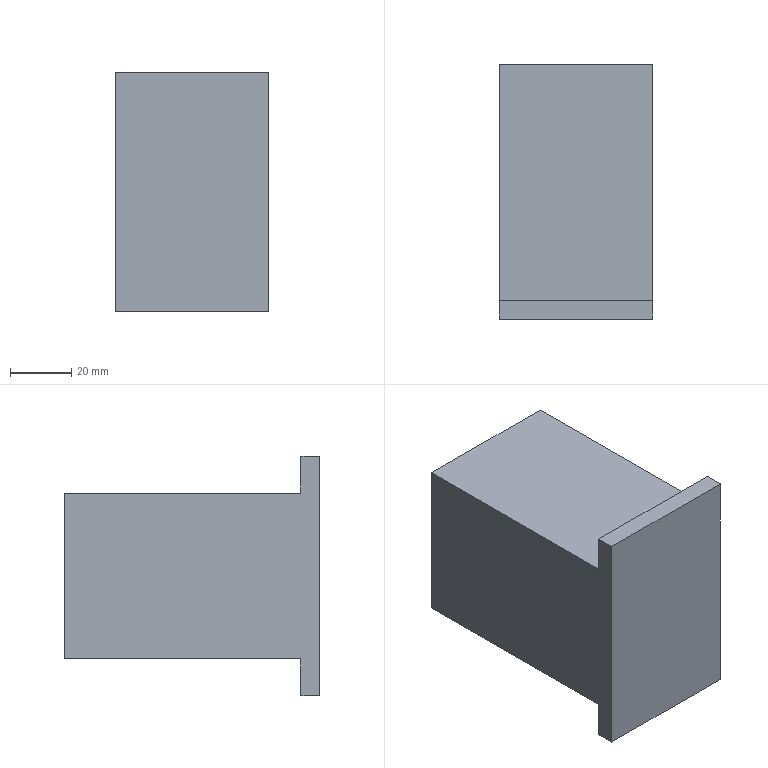Part | SolidWorks | features Extrusion 1, ICE 1 | 1 solid | 10 faces | box 50 x 83 x 78 mm | volume 231300 mm3 | plane 10
STEP:
#1=CARTESIAN_POINT('',(-25.,41.5,27.));
#2=VERTEX_POINT('',#1);
#3=CARTESIAN_POINT('',(-25.,41.5,-27.));
#4=VERTEX_POINT('',#3);
#5=CARTESIAN_POINT('',(-25.,41.5,39.));
#6=DIRECTION('',(0.,0.,-1.));
#7=VECTOR('',#6,1000.);
#8=LINE('',#5,#7);
#9=EDGE_CURVE('',#2,#4,#8,.T.);
#10=ORIENTED_EDGE('',*,*,#9,.T.);
#11=CARTESIAN_POINT('',(-25.,-35.5,-27.));
#12=VERTEX_POINT('',#11);
#13=CARTESIAN_POINT('',(-25.,41.5,-27.));
#14=DIRECTION('',(0.,1.,0.));
#15=VECTOR('',#14,1000.);
#16=LINE('',#13,#15);
#17=EDGE_CURVE('',#12,#4,#16,.T.);
#18=ORIENTED_EDGE('',*,*,#17,.F.);
#19=CARTESIAN_POINT('',(-25.,-35.5,-39.));
#20=VERTEX_POINT('',#19);
#21=CARTESIAN_POINT('',(-25.,-35.5,-39.));
#22=DIRECTION('',(0.,0.,1.));
#23=VECTOR('',#22,1000.);
#24=LINE('',#21,#23);
#25=EDGE_CURVE('',#20,#12,#24,.T.);
#26=ORIENTED_EDGE('',*,*,#25,.F.);
#27=CARTESIAN_POINT('',(-25.,-41.5,-39.));
#28=VERTEX_POINT('',#27);
#29=CARTESIAN_POINT('',(-25.,-41.5,-39.));
#30=DIRECTION('',(0.,-1.,0.));
#31=VECTOR('',#30,1000.);
#32=LINE('',#29,#31);
#33=EDGE_CURVE('',#20,#28,#32,.T.);
#34=ORIENTED_EDGE('',*,*,#33,.T.);
#35=CARTESIAN_POINT('',(-25.,-41.5,39.));
#36=VERTEX_POINT('',#35);
#37=CARTESIAN_POINT('',(-25.,-41.5,39.));
#38=DIRECTION('',(0.,0.,-1.));
#39=VECTOR('',#38,1000.);
#40=LINE('',#37,#39);
#41=EDGE_CURVE('',#36,#28,#40,.T.);
#42=ORIENTED_EDGE('',*,*,#41,.F.);
#43=CARTESIAN_POINT('',(-25.,-35.5,39.));
#44=VERTEX_POINT('',#43);
#45=CARTESIAN_POINT('',(-25.,-41.5,39.));
#46=DIRECTION('',(0.,-1.,0.));
#47=VECTOR('',#46,1000.);
#48=LINE('',#45,#47);
#49=EDGE_CURVE('',#44,#36,#48,.T.);
#50=ORIENTED_EDGE('',*,*,#49,.F.);
#51=CARTESIAN_POINT('',(-25.,-35.5,27.));
#52=VERTEX_POINT('',#51);
#53=CARTESIAN_POINT('',(-25.,-35.5,39.));
#54=DIRECTION('',(0.,0.,1.));
#55=VECTOR('',#54,1000.);
#56=LINE('',#53,#55);
#57=EDGE_CURVE('',#52,#44,#56,.T.);
#58=ORIENTED_EDGE('',*,*,#57,.F.);
#59=CARTESIAN_POINT('',(-25.,41.5,27.));
#60=DIRECTION('',(0.,-1.,0.));
#61=VECTOR('',#60,1000.);
#62=LINE('',#59,#61);
#63=EDGE_CURVE('',#2,#52,#62,.T.);
#64=ORIENTED_EDGE('',*,*,#63,.F.);
#65=EDGE_LOOP('',(#10,#18,#26,#34,#42,#50,#58,#64));
#66=FACE_OUTER_BOUND('',#65,.T.);
#67=CARTESIAN_POINT('',(-25.,-41.5,39.));
#68=DIRECTION('',(1.,0.,0.));
#69=DIRECTION('',(0.,0.,-1.));
#70=AXIS2_PLACEMENT_3D('',#67,#68,#69);
#71=PLANE('',#70);
#72=ADVANCED_FACE('',(#66),#71,.F.);
#73=CARTESIAN_POINT('',(25.,-41.5,-39.));
#74=VERTEX_POINT('',#73);
#75=CARTESIAN_POINT('',(25.,-41.5,-39.));
#76=DIRECTION('',(1.,0.,0.));
#77=VECTOR('',#76,1000.);
#78=LINE('',#75,#77);
#79=EDGE_CURVE('',#28,#74,#78,.T.);
#80=ORIENTED_EDGE('',*,*,#79,.T.);
#81=CARTESIAN_POINT('',(25.,-41.5,39.));
#82=VERTEX_POINT('',#81);
#83=CARTESIAN_POINT('',(25.,-41.5,39.));
#84=DIRECTION('',(0.,0.,-1.));
#85=VECTOR('',#84,1000.);
#86=LINE('',#83,#85);
#87=EDGE_CURVE('',#82,#74,#86,.T.);
#88=ORIENTED_EDGE('',*,*,#87,.F.);
#89=CARTESIAN_POINT('',(25.,-41.5,39.));
#90=DIRECTION('',(1.,0.,0.));
#91=VECTOR('',#90,1000.);
#92=LINE('',#89,#91);
#93=EDGE_CURVE('',#36,#82,#92,.T.);
#94=ORIENTED_EDGE('',*,*,#93,.F.);
#95=ORIENTED_EDGE('',*,*,#41,.T.);
#96=EDGE_LOOP('',(#80,#88,#94,#95));
#97=FACE_OUTER_BOUND('',#96,.T.);
#98=CARTESIAN_POINT('',(25.,-41.5,39.));
#99=DIRECTION('',(0.,1.,0.));
#100=DIRECTION('',(0.,0.,1.));
#101=AXIS2_PLACEMENT_3D('',#98,#99,#100);
#102=PLANE('',#101);
#103=ADVANCED_FACE('',(#97),#102,.F.);
#104=CARTESIAN_POINT('',(25.,-35.5,-39.));
#105=VERTEX_POINT('',#104);
#106=CARTESIAN_POINT('',(25.,-35.5,-27.));
#107=VERTEX_POINT('',#106);
#108=CARTESIAN_POINT('',(25.,-35.5,-39.));
#109=DIRECTION('',(0.,0.,1.));
#110=VECTOR('',#109,1000.);
#111=LINE('',#108,#110);
#112=EDGE_CURVE('',#105,#107,#111,.T.);
#113=ORIENTED_EDGE('',*,*,#112,.T.);
#114=CARTESIAN_POINT('',(25.,41.5,-27.));
#115=VERTEX_POINT('',#114);
#116=CARTESIAN_POINT('',(25.,41.5,-27.));
#117=DIRECTION('',(0.,1.,0.));
#118=VECTOR('',#117,1000.);
#119=LINE('',#116,#118);
#120=EDGE_CURVE('',#107,#115,#119,.T.);
#121=ORIENTED_EDGE('',*,*,#120,.T.);
#122=CARTESIAN_POINT('',(25.,41.5,27.));
#123=VERTEX_POINT('',#122);
#124=CARTESIAN_POINT('',(25.,41.5,39.));
#125=DIRECTION('',(0.,0.,-1.));
#126=VECTOR('',#125,1000.);
#127=LINE('',#124,#126);
#128=EDGE_CURVE('',#123,#115,#127,.T.);
#129=ORIENTED_EDGE('',*,*,#128,.F.);
#130=CARTESIAN_POINT('',(25.,-35.5,27.));
#131=VERTEX_POINT('',#130);
#132=CARTESIAN_POINT('',(25.,41.5,27.));
#133=DIRECTION('',(0.,-1.,0.));
#134=VECTOR('',#133,1000.);
#135=LINE('',#132,#134);
#136=EDGE_CURVE('',#123,#131,#135,.T.);
#137=ORIENTED_EDGE('',*,*,#136,.T.);
#138=CARTESIAN_POINT('',(25.,-35.5,39.));
#139=VERTEX_POINT('',#138);
#140=CARTESIAN_POINT('',(25.,-35.5,39.));
#141=DIRECTION('',(0.,0.,1.));
#142=VECTOR('',#141,1000.);
#143=LINE('',#140,#142);
#144=EDGE_CURVE('',#131,#139,#143,.T.);
#145=ORIENTED_EDGE('',*,*,#144,.T.);
#146=CARTESIAN_POINT('',(25.,-41.5,39.));
#147=DIRECTION('',(0.,1.,0.));
#148=VECTOR('',#147,1000.);
#149=LINE('',#146,#148);
#150=EDGE_CURVE('',#82,#139,#149,.T.);
#151=ORIENTED_EDGE('',*,*,#150,.F.);
#152=ORIENTED_EDGE('',*,*,#87,.T.);
#153=CARTESIAN_POINT('',(25.,-41.5,-39.));
#154=DIRECTION('',(0.,1.,0.));
#155=VECTOR('',#154,1000.);
#156=LINE('',#153,#155);
#157=EDGE_CURVE('',#74,#105,#156,.T.);
#158=ORIENTED_EDGE('',*,*,#157,.T.);
#159=EDGE_LOOP('',(#113,#121,#129,#137,#145,#151,#152,#158));
#160=FACE_OUTER_BOUND('',#159,.T.);
#161=CARTESIAN_POINT('',(25.,-41.5,39.));
#162=DIRECTION('',(-1.,0.,0.));
#163=DIRECTION('',(0.,0.,1.));
#164=AXIS2_PLACEMENT_3D('',#161,#162,#163);
#165=PLANE('',#164);
#166=ADVANCED_FACE('',(#160),#165,.F.);
#167=ORIENTED_EDGE('',*,*,#128,.T.);
#168=CARTESIAN_POINT('',(25.,41.5,-27.));
#169=DIRECTION('',(-1.,0.,0.));
#170=VECTOR('',#169,1000.);
#171=LINE('',#168,#170);
#172=EDGE_CURVE('',#115,#4,#171,.T.);
#173=ORIENTED_EDGE('',*,*,#172,.T.);
#174=ORIENTED_EDGE('',*,*,#9,.F.);
#175=CARTESIAN_POINT('',(25.,41.5,27.));
#176=DIRECTION('',(-1.,0.,0.));
#177=VECTOR('',#176,1000.);
#178=LINE('',#175,#177);
#179=EDGE_CURVE('',#123,#2,#178,.T.);
#180=ORIENTED_EDGE('',*,*,#179,.F.);
#181=EDGE_LOOP('',(#167,#173,#174,#180));
#182=FACE_OUTER_BOUND('',#181,.T.);
#183=CARTESIAN_POINT('',(25.,41.5,39.));
#184=DIRECTION('',(0.,-1.,0.));
#185=DIRECTION('',(1.,0.,0.));
#186=AXIS2_PLACEMENT_3D('',#183,#184,#185);
#187=PLANE('',#186);
#188=ADVANCED_FACE('',(#182),#187,.F.);
#189=CARTESIAN_POINT('',(25.,-35.5,39.));
#190=DIRECTION('',(-1.,0.,0.));
#191=VECTOR('',#190,1000.);
#192=LINE('',#189,#191);
#193=EDGE_CURVE('',#139,#44,#192,.T.);
#194=ORIENTED_EDGE('',*,*,#193,.T.);
#195=ORIENTED_EDGE('',*,*,#49,.T.);
#196=ORIENTED_EDGE('',*,*,#93,.T.);
#197=ORIENTED_EDGE('',*,*,#150,.T.);
#198=EDGE_LOOP('',(#194,#195,#196,#197));
#199=FACE_OUTER_BOUND('',#198,.T.);
#200=CARTESIAN_POINT('',(0.,0.,39.));
#201=DIRECTION('',(0.,0.,1.));
#202=DIRECTION('',(1.,0.,0.));
#203=AXIS2_PLACEMENT_3D('',#200,#201,#202);
#204=PLANE('',#203);
#205=ADVANCED_FACE('',(#199),#204,.T.);
#206=ORIENTED_EDGE('',*,*,#33,.F.);
#207=CARTESIAN_POINT('',(25.,-35.5,-39.));
#208=DIRECTION('',(-1.,0.,0.));
#209=VECTOR('',#208,1000.);
#210=LINE('',#207,#209);
#211=EDGE_CURVE('',#105,#20,#210,.T.);
#212=ORIENTED_EDGE('',*,*,#211,.F.);
#213=ORIENTED_EDGE('',*,*,#157,.F.);
#214=ORIENTED_EDGE('',*,*,#79,.F.);
#215=EDGE_LOOP('',(#206,#212,#213,#214));
#216=FACE_OUTER_BOUND('',#215,.T.);
#217=CARTESIAN_POINT('',(0.,0.,-39.));
#218=DIRECTION('',(0.,0.,1.));
#219=DIRECTION('',(1.,0.,0.));
#220=AXIS2_PLACEMENT_3D('',#217,#218,#219);
#221=PLANE('',#220);
#222=ADVANCED_FACE('',(#216),#221,.F.);
#223=ORIENTED_EDGE('',*,*,#17,.T.);
#224=ORIENTED_EDGE('',*,*,#172,.F.);
#225=ORIENTED_EDGE('',*,*,#120,.F.);
#226=CARTESIAN_POINT('',(25.,-35.5,-27.));
#227=DIRECTION('',(-1.,0.,0.));
#228=VECTOR('',#227,1000.);
#229=LINE('',#226,#228);
#230=EDGE_CURVE('',#107,#12,#229,.T.);
#231=ORIENTED_EDGE('',*,*,#230,.T.);
#232=EDGE_LOOP('',(#223,#224,#225,#231));
#233=FACE_OUTER_BOUND('',#232,.T.);
#234=CARTESIAN_POINT('',(25.,41.5,-27.));
#235=DIRECTION('',(0.,0.,1.));
#236=DIRECTION('',(0.,-1.,0.));
#237=AXIS2_PLACEMENT_3D('',#234,#235,#236);
#238=PLANE('',#237);
#239=ADVANCED_FACE('',(#233),#238,.F.);
#240=ORIENTED_EDGE('',*,*,#25,.T.);
#241=ORIENTED_EDGE('',*,*,#230,.F.);
#242=ORIENTED_EDGE('',*,*,#112,.F.);
#243=ORIENTED_EDGE('',*,*,#211,.T.);
#244=EDGE_LOOP('',(#240,#241,#242,#243));
#245=FACE_OUTER_BOUND('',#244,.T.);
#246=CARTESIAN_POINT('',(25.,-35.5,-39.));
#247=DIRECTION('',(0.,-1.,0.));
#248=DIRECTION('',(0.,0.,-1.));
#249=AXIS2_PLACEMENT_3D('',#246,#247,#248);
#250=PLANE('',#249);
#251=ADVANCED_FACE('',(#245),#250,.F.);
#252=ORIENTED_EDGE('',*,*,#57,.T.);
#253=ORIENTED_EDGE('',*,*,#193,.F.);
#254=ORIENTED_EDGE('',*,*,#144,.F.);
#255=CARTESIAN_POINT('',(25.,-35.5,27.));
#256=DIRECTION('',(-1.,0.,0.));
#257=VECTOR('',#256,1000.);
#258=LINE('',#255,#257);
#259=EDGE_CURVE('',#131,#52,#258,.T.);
#260=ORIENTED_EDGE('',*,*,#259,.T.);
#261=EDGE_LOOP('',(#252,#253,#254,#260));
#262=FACE_OUTER_BOUND('',#261,.T.);
#263=CARTESIAN_POINT('',(25.,-35.5,39.));
#264=DIRECTION('',(0.,-1.,0.));
#265=DIRECTION('',(0.,0.,-1.));
#266=AXIS2_PLACEMENT_3D('',#263,#264,#265);
#267=PLANE('',#266);
#268=ADVANCED_FACE('',(#262),#267,.F.);
#269=ORIENTED_EDGE('',*,*,#63,.T.);
#270=ORIENTED_EDGE('',*,*,#259,.F.);
#271=ORIENTED_EDGE('',*,*,#136,.F.);
#272=ORIENTED_EDGE('',*,*,#179,.T.);
#273=EDGE_LOOP('',(#269,#270,#271,#272));
#274=FACE_OUTER_BOUND('',#273,.T.);
#275=CARTESIAN_POINT('',(25.,41.5,27.));
#276=DIRECTION('',(0.,0.,-1.));
#277=DIRECTION('',(0.,1.,0.));
#278=AXIS2_PLACEMENT_3D('',#275,#276,#277);
#279=PLANE('',#278);
#280=ADVANCED_FACE('',(#274),#279,.F.);
#281=CLOSED_SHELL('',(#72,#103,#166,#188,#205,#222,#239,#251,#268,#280));
#282=MANIFOLD_SOLID_BREP('',#281);
#283=CARTESIAN_POINT('',(0.,0.,0.));
#284=DIRECTION('',(0.,0.,1.));
#285=DIRECTION('',(1.,0.,0.));
#286=AXIS2_PLACEMENT_3D('',#283,#284,#285);
#287=(LENGTH_UNIT()NAMED_UNIT(*)SI_UNIT(.MILLI.,.METRE.));
#288=UNCERTAINTY_MEASURE_WITH_UNIT(LENGTH_MEASURE(0.00001),#287,'','');
#289=(NAMED_UNIT(*)PLANE_ANGLE_UNIT()SI_UNIT($,.RADIAN.));
#290=(NAMED_UNIT(*)SI_UNIT($,.STERADIAN.)SOLID_ANGLE_UNIT());
#291=(GEOMETRIC_REPRESENTATION_CONTEXT(3)GLOBAL_UNCERTAINTY_ASSIGNED_CONTEXT((#288))GLOBAL_UNIT_ASSIGNED_CONTEXT((#287,#289,#290))REPRESENTATION_CONTEXT('',''));
#292=ADVANCED_BREP_SHAPE_REPRESENTATION('',(#282,#286),#291);